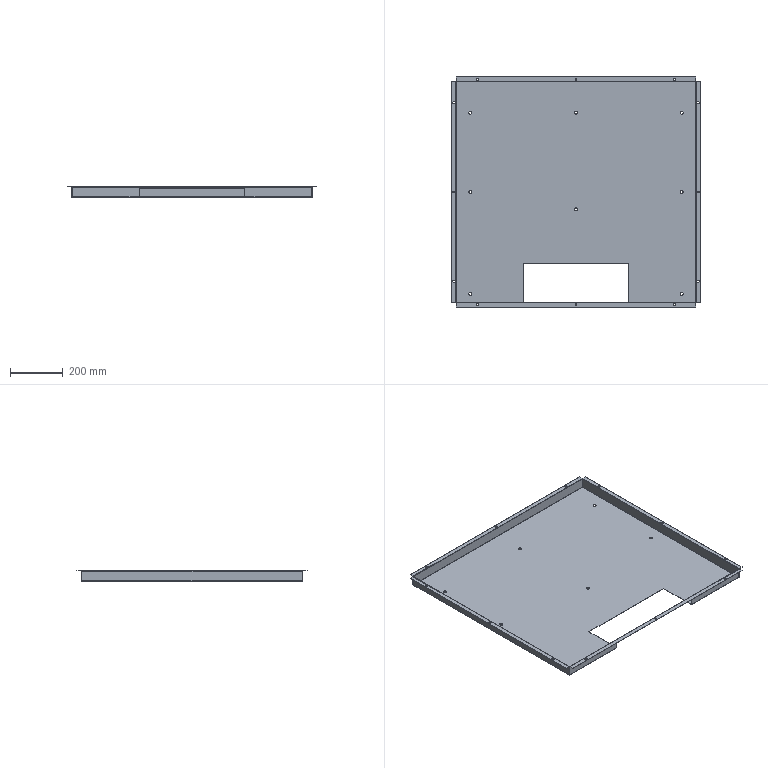Part | 1 solid | 150 faces | box 940 x 870 x 40 mm | volume 876610 mm3 | plane 78 | cylinder 64 | spline 8 | commonest cylinder face diameters 7 x30 11 x16 0.4 x9 2.4 x9